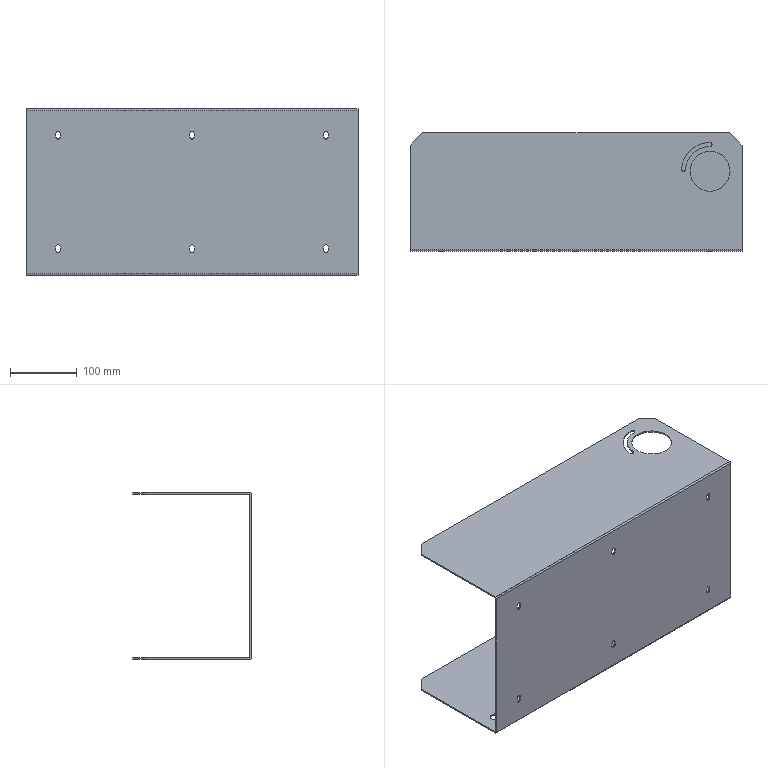Part | STEP file | Control Box Lower Base 1 | 1 solid | 57 faces | box 498 x 178 x 250 mm | volume 589659 mm3 | cylinder 31 | plane 26 | commonest cylinder face diameters 6.5 x18 6 x3 0.2 x2 4.2 x2 15 x2 60 x2